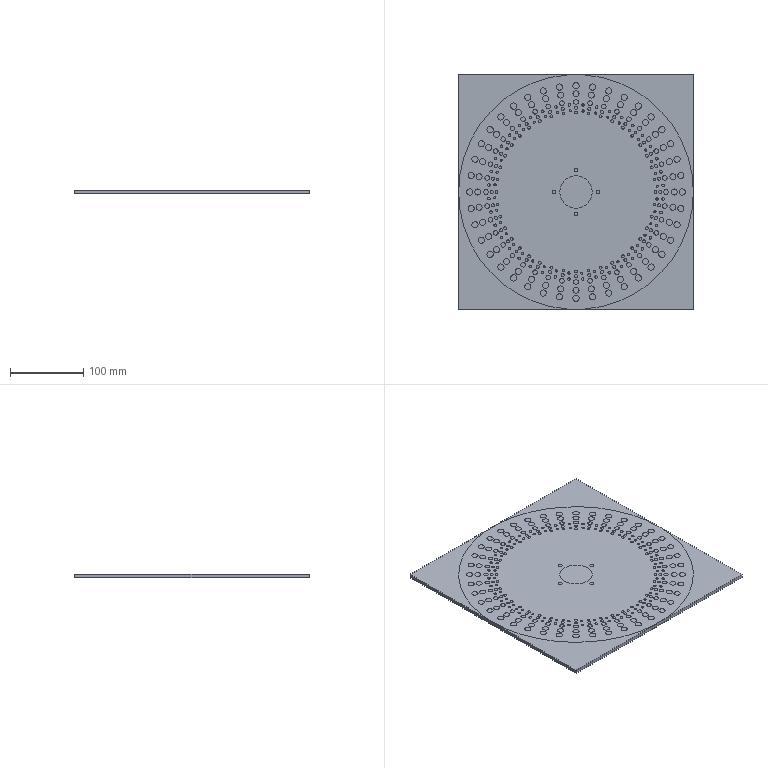Part | 2 solids | 294 faces | box 320 x 320 x 5 mm | volume 869887 mm3 | cylinder 286 | plane 8 | commonest cylinder face diameters 3 x40 3.5 x40 3.9 x40 4 x40 6.2 x40 8.2 x40